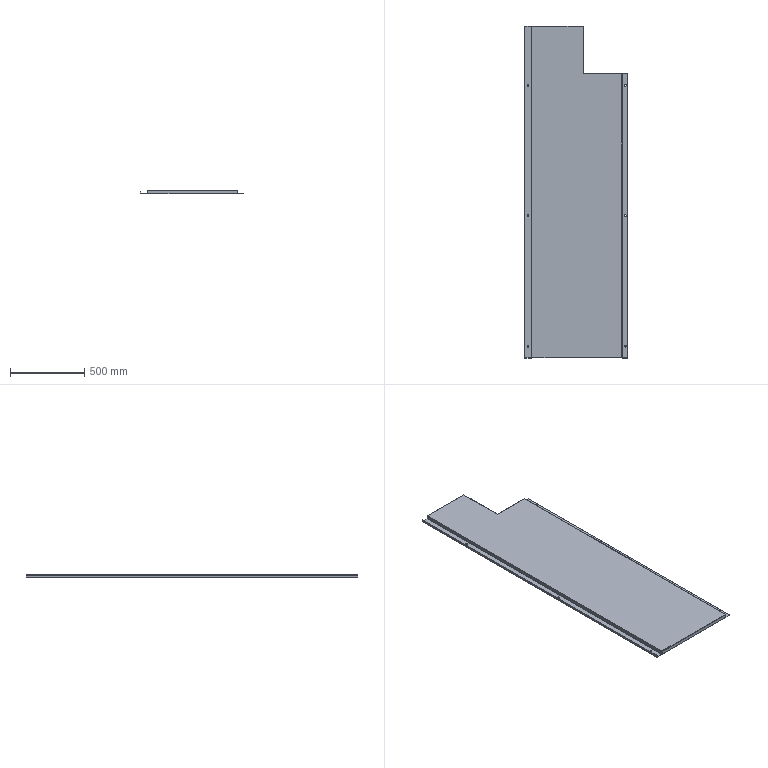Part | STEP file | 1 solid | 92 faces | box 697 x 2240 x 25 mm | volume 2428622 mm3 | plane 50 | cylinder 30 | spline 12 | commonest cylinder face diameters 12 x12 2 x9 5 x9